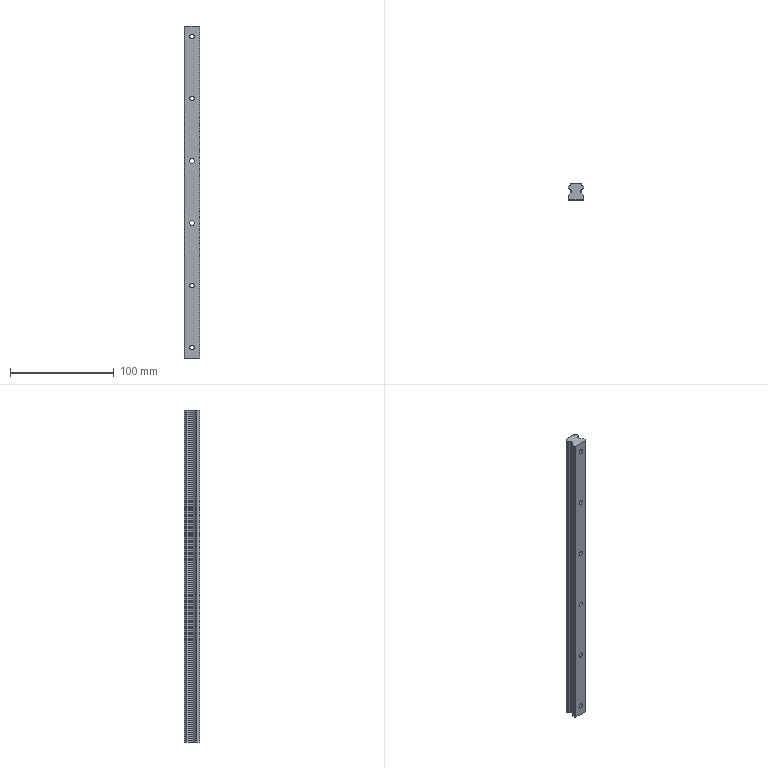Part | NX | features BREP 1 | 1 solid | 66 faces | box 15 x 15 x 320 mm | volume 58712 mm3 | cylinder 38 | plane 28 | commonest cylinder face diameters 4.5 x12 7.5 x12 0.8 x8 3.24 x4 2 x2